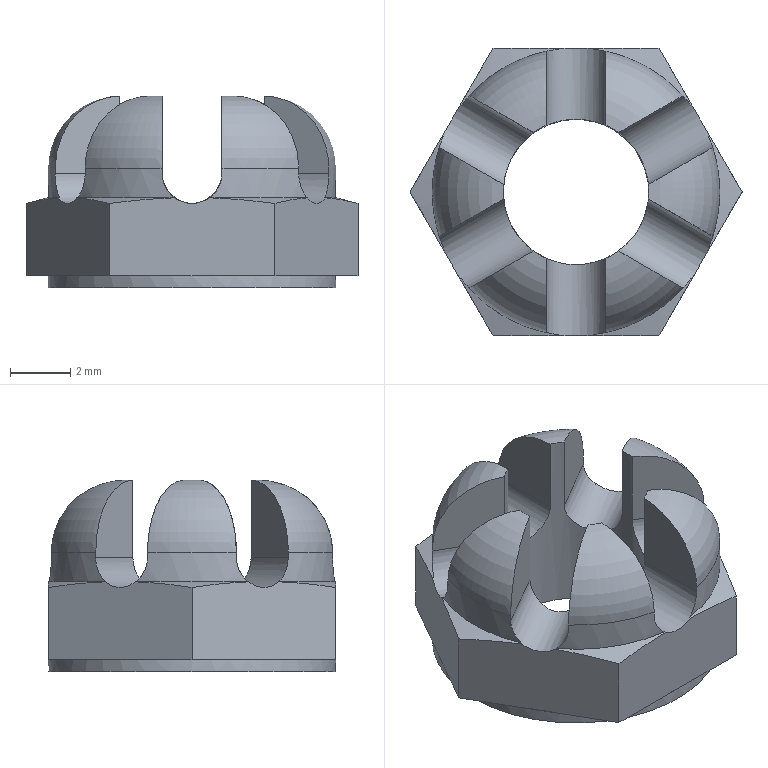Part | NX | features solid 2 | 1 solid | 51 faces | box 10.999 x 9.525 x 6.35 mm | volume 242.081 mm3 | plane 25 | cylinder 14 | torus 6 | cone 6 | commonest cylinder face diameters 9.525 x7 1.984 x6 4.826 x1